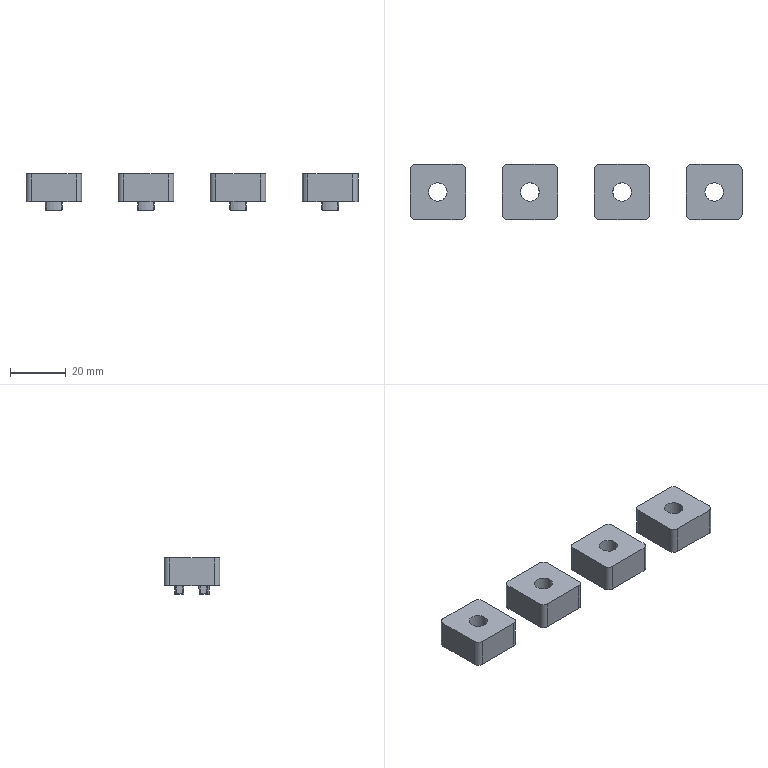Part | 4 solids | 144 faces | box 118.91 x 19.91 x 13 mm | volume 14714 mm3 | plane 80 | cylinder 40 | spline 16 | cone 8 | commonest cylinder face diameters 1 x16 3.91 x16 6.6 x8